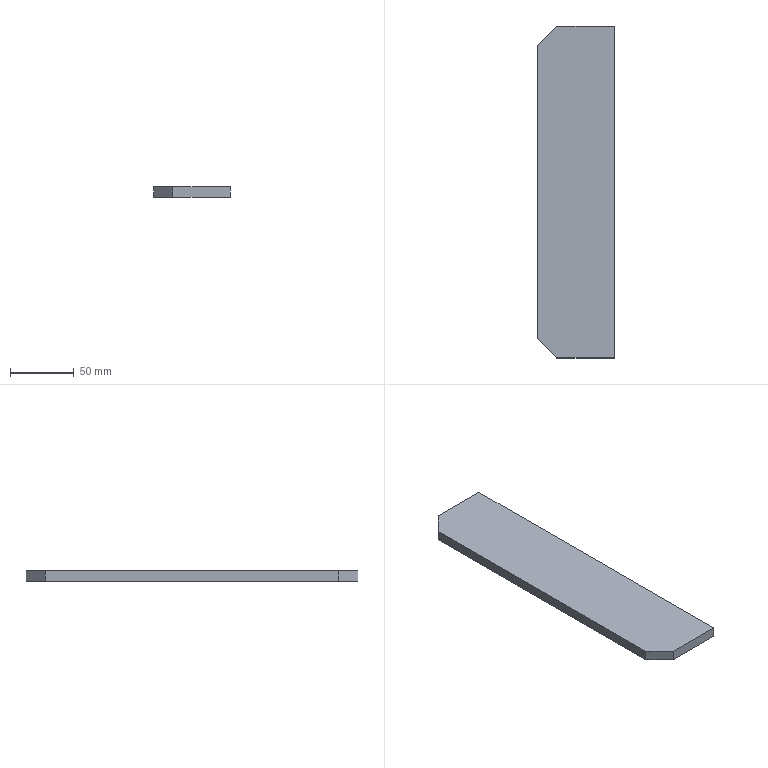Part | SolidWorks | features Chamfer 1, Extrusion 1 | 1 solid | 8 faces | box 60 x 260 x 8 mm | volume 123000 mm3 | plane 8
STEP:
#1=CARTESIAN_POINT('',(-30.,115.,0.));
#2=VERTEX_POINT('',#1);
#3=CARTESIAN_POINT('',(-30.,-115.,0.));
#4=VERTEX_POINT('',#3);
#5=CARTESIAN_POINT('',(-30.,-130.,0.));
#6=DIRECTION('',(0.,-1.,0.));
#7=VECTOR('',#6,1000.);
#8=LINE('',#5,#7);
#9=EDGE_CURVE('',#2,#4,#8,.T.);
#10=ORIENTED_EDGE('',*,*,#9,.T.);
#11=CARTESIAN_POINT('',(-30.,-115.,8.));
#12=VERTEX_POINT('',#11);
#13=CARTESIAN_POINT('',(-30.,-115.,8.));
#14=DIRECTION('',(0.,0.,1.));
#15=VECTOR('',#14,1000.);
#16=LINE('',#13,#15);
#17=EDGE_CURVE('',#4,#12,#16,.T.);
#18=ORIENTED_EDGE('',*,*,#17,.T.);
#19=CARTESIAN_POINT('',(-30.,115.,8.));
#20=VERTEX_POINT('',#19);
#21=CARTESIAN_POINT('',(-30.,-130.,8.));
#22=DIRECTION('',(0.,-1.,0.));
#23=VECTOR('',#22,1000.);
#24=LINE('',#21,#23);
#25=EDGE_CURVE('',#20,#12,#24,.T.);
#26=ORIENTED_EDGE('',*,*,#25,.F.);
#27=CARTESIAN_POINT('',(-30.,115.,8.));
#28=DIRECTION('',(0.,0.,-1.));
#29=VECTOR('',#28,1000.);
#30=LINE('',#27,#29);
#31=EDGE_CURVE('',#20,#2,#30,.T.);
#32=ORIENTED_EDGE('',*,*,#31,.T.);
#33=EDGE_LOOP('',(#10,#18,#26,#32));
#34=FACE_OUTER_BOUND('',#33,.T.);
#35=CARTESIAN_POINT('',(-30.,-130.,8.));
#36=DIRECTION('',(1.,0.,0.));
#37=DIRECTION('',(0.,0.,-1.));
#38=AXIS2_PLACEMENT_3D('',#35,#36,#37);
#39=PLANE('',#38);
#40=ADVANCED_FACE('',(#34),#39,.F.);
#41=CARTESIAN_POINT('',(-15.,-130.,8.));
#42=VERTEX_POINT('',#41);
#43=CARTESIAN_POINT('',(30.,-130.,8.));
#44=VERTEX_POINT('',#43);
#45=CARTESIAN_POINT('',(30.,-130.,8.));
#46=DIRECTION('',(1.,0.,0.));
#47=VECTOR('',#46,1000.);
#48=LINE('',#45,#47);
#49=EDGE_CURVE('',#42,#44,#48,.T.);
#50=ORIENTED_EDGE('',*,*,#49,.F.);
#51=CARTESIAN_POINT('',(-15.,-130.,0.));
#52=VERTEX_POINT('',#51);
#53=CARTESIAN_POINT('',(-15.,-130.,8.));
#54=DIRECTION('',(0.,0.,-1.));
#55=VECTOR('',#54,1000.);
#56=LINE('',#53,#55);
#57=EDGE_CURVE('',#42,#52,#56,.T.);
#58=ORIENTED_EDGE('',*,*,#57,.T.);
#59=CARTESIAN_POINT('',(30.,-130.,0.));
#60=VERTEX_POINT('',#59);
#61=CARTESIAN_POINT('',(30.,-130.,0.));
#62=DIRECTION('',(1.,0.,0.));
#63=VECTOR('',#62,1000.);
#64=LINE('',#61,#63);
#65=EDGE_CURVE('',#52,#60,#64,.T.);
#66=ORIENTED_EDGE('',*,*,#65,.T.);
#67=CARTESIAN_POINT('',(30.,-130.,8.));
#68=DIRECTION('',(0.,0.,-1.));
#69=VECTOR('',#68,1000.);
#70=LINE('',#67,#69);
#71=EDGE_CURVE('',#44,#60,#70,.T.);
#72=ORIENTED_EDGE('',*,*,#71,.F.);
#73=EDGE_LOOP('',(#50,#58,#66,#72));
#74=FACE_OUTER_BOUND('',#73,.T.);
#75=CARTESIAN_POINT('',(30.,-130.,8.));
#76=DIRECTION('',(0.,1.,0.));
#77=DIRECTION('',(0.,0.,1.));
#78=AXIS2_PLACEMENT_3D('',#75,#76,#77);
#79=PLANE('',#78);
#80=ADVANCED_FACE('',(#74),#79,.F.);
#81=CARTESIAN_POINT('',(30.,130.,0.));
#82=VERTEX_POINT('',#81);
#83=CARTESIAN_POINT('',(30.,-130.,0.));
#84=DIRECTION('',(0.,1.,0.));
#85=VECTOR('',#84,1000.);
#86=LINE('',#83,#85);
#87=EDGE_CURVE('',#60,#82,#86,.T.);
#88=ORIENTED_EDGE('',*,*,#87,.T.);
#89=CARTESIAN_POINT('',(30.,130.,8.));
#90=VERTEX_POINT('',#89);
#91=CARTESIAN_POINT('',(30.,130.,8.));
#92=DIRECTION('',(0.,0.,-1.));
#93=VECTOR('',#92,1000.);
#94=LINE('',#91,#93);
#95=EDGE_CURVE('',#90,#82,#94,.T.);
#96=ORIENTED_EDGE('',*,*,#95,.F.);
#97=CARTESIAN_POINT('',(30.,-130.,8.));
#98=DIRECTION('',(0.,1.,0.));
#99=VECTOR('',#98,1000.);
#100=LINE('',#97,#99);
#101=EDGE_CURVE('',#44,#90,#100,.T.);
#102=ORIENTED_EDGE('',*,*,#101,.F.);
#103=ORIENTED_EDGE('',*,*,#71,.T.);
#104=EDGE_LOOP('',(#88,#96,#102,#103));
#105=FACE_OUTER_BOUND('',#104,.T.);
#106=CARTESIAN_POINT('',(30.,-130.,8.));
#107=DIRECTION('',(-1.,0.,0.));
#108=DIRECTION('',(0.,0.,1.));
#109=AXIS2_PLACEMENT_3D('',#106,#107,#108);
#110=PLANE('',#109);
#111=ADVANCED_FACE('',(#105),#110,.F.);
#112=CARTESIAN_POINT('',(-15.,130.,0.));
#113=VERTEX_POINT('',#112);
#114=CARTESIAN_POINT('',(30.,130.,0.));
#115=DIRECTION('',(-1.,0.,0.));
#116=VECTOR('',#115,1000.);
#117=LINE('',#114,#116);
#118=EDGE_CURVE('',#82,#113,#117,.T.);
#119=ORIENTED_EDGE('',*,*,#118,.T.);
#120=CARTESIAN_POINT('',(-15.,130.,8.));
#121=VERTEX_POINT('',#120);
#122=CARTESIAN_POINT('',(-15.,130.,8.));
#123=DIRECTION('',(0.,0.,1.));
#124=VECTOR('',#123,1000.);
#125=LINE('',#122,#124);
#126=EDGE_CURVE('',#113,#121,#125,.T.);
#127=ORIENTED_EDGE('',*,*,#126,.T.);
#128=CARTESIAN_POINT('',(30.,130.,8.));
#129=DIRECTION('',(-1.,0.,0.));
#130=VECTOR('',#129,1000.);
#131=LINE('',#128,#130);
#132=EDGE_CURVE('',#90,#121,#131,.T.);
#133=ORIENTED_EDGE('',*,*,#132,.F.);
#134=ORIENTED_EDGE('',*,*,#95,.T.);
#135=EDGE_LOOP('',(#119,#127,#133,#134));
#136=FACE_OUTER_BOUND('',#135,.T.);
#137=CARTESIAN_POINT('',(30.,130.,8.));
#138=DIRECTION('',(0.,-1.,0.));
#139=DIRECTION('',(0.,0.,-1.));
#140=AXIS2_PLACEMENT_3D('',#137,#138,#139);
#141=PLANE('',#140);
#142=ADVANCED_FACE('',(#136),#141,.F.);
#143=ORIENTED_EDGE('',*,*,#25,.T.);
#144=CARTESIAN_POINT('',(-72.5,-72.5,8.));
#145=DIRECTION('',(0.7071,-0.7071,0.));
#146=VECTOR('',#145,1000.);
#147=LINE('',#144,#146);
#148=EDGE_CURVE('',#12,#42,#147,.T.);
#149=ORIENTED_EDGE('',*,*,#148,.T.);
#150=ORIENTED_EDGE('',*,*,#49,.T.);
#151=ORIENTED_EDGE('',*,*,#101,.T.);
#152=ORIENTED_EDGE('',*,*,#132,.T.);
#153=CARTESIAN_POINT('',(-72.5,72.5,8.));
#154=DIRECTION('',(-0.7071,-0.7071,0.));
#155=VECTOR('',#154,1000.);
#156=LINE('',#153,#155);
#157=EDGE_CURVE('',#121,#20,#156,.T.);
#158=ORIENTED_EDGE('',*,*,#157,.T.);
#159=EDGE_LOOP('',(#143,#149,#150,#151,#152,#158));
#160=FACE_OUTER_BOUND('',#159,.T.);
#161=CARTESIAN_POINT('',(0.,0.,8.));
#162=DIRECTION('',(0.,0.,1.));
#163=DIRECTION('',(1.,0.,0.));
#164=AXIS2_PLACEMENT_3D('',#161,#162,#163);
#165=PLANE('',#164);
#166=ADVANCED_FACE('',(#160),#165,.T.);
#167=ORIENTED_EDGE('',*,*,#65,.F.);
#168=CARTESIAN_POINT('',(-15.,-130.,0.));
#169=DIRECTION('',(-0.7071,0.7071,0.));
#170=VECTOR('',#169,1000.);
#171=LINE('',#168,#170);
#172=EDGE_CURVE('',#52,#4,#171,.T.);
#173=ORIENTED_EDGE('',*,*,#172,.T.);
#174=ORIENTED_EDGE('',*,*,#9,.F.);
#175=CARTESIAN_POINT('',(-30.,115.,0.));
#176=DIRECTION('',(0.7071,0.7071,0.));
#177=VECTOR('',#176,1000.);
#178=LINE('',#175,#177);
#179=EDGE_CURVE('',#2,#113,#178,.T.);
#180=ORIENTED_EDGE('',*,*,#179,.T.);
#181=ORIENTED_EDGE('',*,*,#118,.F.);
#182=ORIENTED_EDGE('',*,*,#87,.F.);
#183=EDGE_LOOP('',(#167,#173,#174,#180,#181,#182));
#184=FACE_OUTER_BOUND('',#183,.T.);
#185=CARTESIAN_POINT('',(0.,0.,0.));
#186=DIRECTION('',(0.,0.,1.));
#187=DIRECTION('',(1.,0.,0.));
#188=AXIS2_PLACEMENT_3D('',#185,#186,#187);
#189=PLANE('',#188);
#190=ADVANCED_FACE('',(#184),#189,.F.);
#191=ORIENTED_EDGE('',*,*,#148,.F.);
#192=ORIENTED_EDGE('',*,*,#17,.F.);
#193=ORIENTED_EDGE('',*,*,#172,.F.);
#194=ORIENTED_EDGE('',*,*,#57,.F.);
#195=EDGE_LOOP('',(#191,#192,#193,#194));
#196=FACE_OUTER_BOUND('',#195,.T.);
#197=CARTESIAN_POINT('',(-15.,-130.,8.));
#198=DIRECTION('',(0.7071,0.7071,0.));
#199=DIRECTION('',(0.,0.,-1.));
#200=AXIS2_PLACEMENT_3D('',#197,#198,#199);
#201=PLANE('',#200);
#202=ADVANCED_FACE('',(#196),#201,.F.);
#203=ORIENTED_EDGE('',*,*,#157,.F.);
#204=ORIENTED_EDGE('',*,*,#126,.F.);
#205=ORIENTED_EDGE('',*,*,#179,.F.);
#206=ORIENTED_EDGE('',*,*,#31,.F.);
#207=EDGE_LOOP('',(#203,#204,#205,#206));
#208=FACE_OUTER_BOUND('',#207,.T.);
#209=CARTESIAN_POINT('',(-30.,115.,8.));
#210=DIRECTION('',(0.7071,-0.7071,0.));
#211=DIRECTION('',(0.,0.,-1.));
#212=AXIS2_PLACEMENT_3D('',#209,#210,#211);
#213=PLANE('',#212);
#214=ADVANCED_FACE('',(#208),#213,.F.);
#215=CLOSED_SHELL('',(#40,#80,#111,#142,#166,#190,#202,#214));
#216=MANIFOLD_SOLID_BREP('',#215);
#217=CARTESIAN_POINT('',(0.,0.,0.));
#218=DIRECTION('',(0.,0.,1.));
#219=DIRECTION('',(1.,0.,0.));
#220=AXIS2_PLACEMENT_3D('',#217,#218,#219);
#221=(LENGTH_UNIT()NAMED_UNIT(*)SI_UNIT(.MILLI.,.METRE.));
#222=UNCERTAINTY_MEASURE_WITH_UNIT(LENGTH_MEASURE(0.00001),#221,'','');
#223=(NAMED_UNIT(*)PLANE_ANGLE_UNIT()SI_UNIT($,.RADIAN.));
#224=(NAMED_UNIT(*)SI_UNIT($,.STERADIAN.)SOLID_ANGLE_UNIT());
#225=(GEOMETRIC_REPRESENTATION_CONTEXT(3)GLOBAL_UNCERTAINTY_ASSIGNED_CONTEXT((#222))GLOBAL_UNIT_ASSIGNED_CONTEXT((#221,#223,#224))REPRESENTATION_CONTEXT('',''));
#226=ADVANCED_BREP_SHAPE_REPRESENTATION('',(#216,#220),#225);